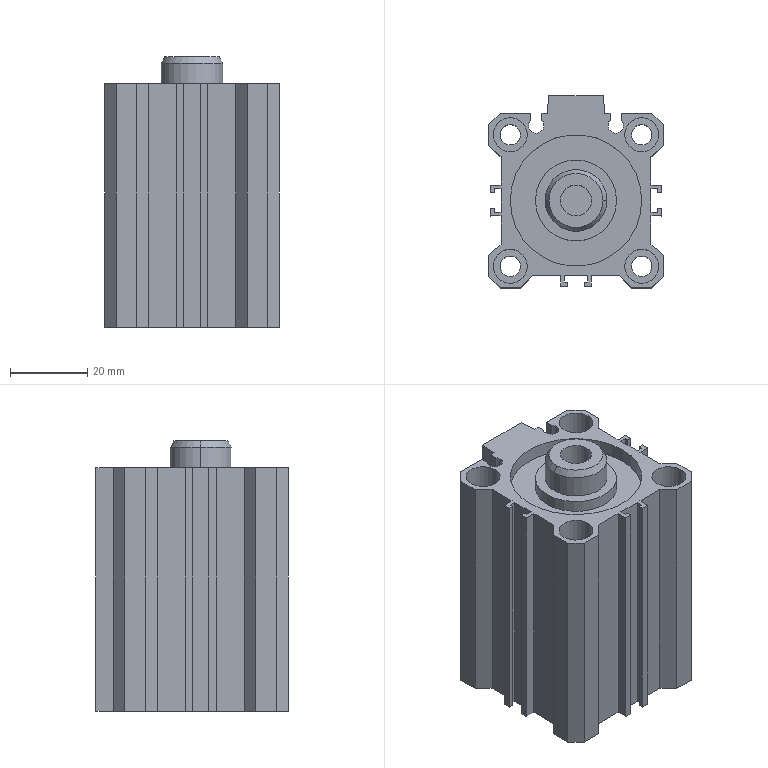Part | STEP file | Air Cylinder CQ2B32-50D | 1 solid | 145 faces | box 45.2 x 49.7 x 70 mm | volume 103939 mm3 | plane 95 | cylinder 44 | cone 6 | commonest cylinder face diameters 8.8 x16 5.3 x8 4 x6 8.5 x4 8 x2 16 x2